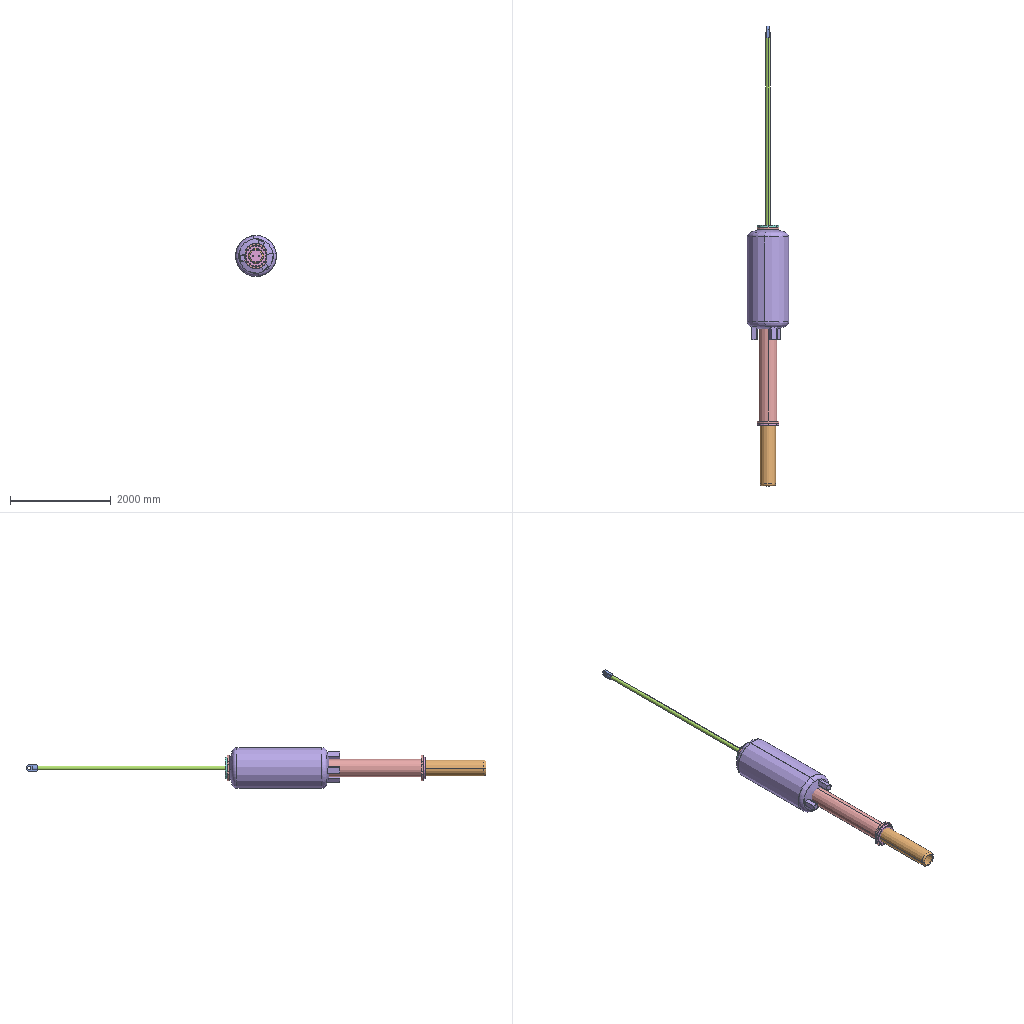Assembly | SolidWorks | 8 different items | 8 placed | box 820 x 9150 x 811 mm
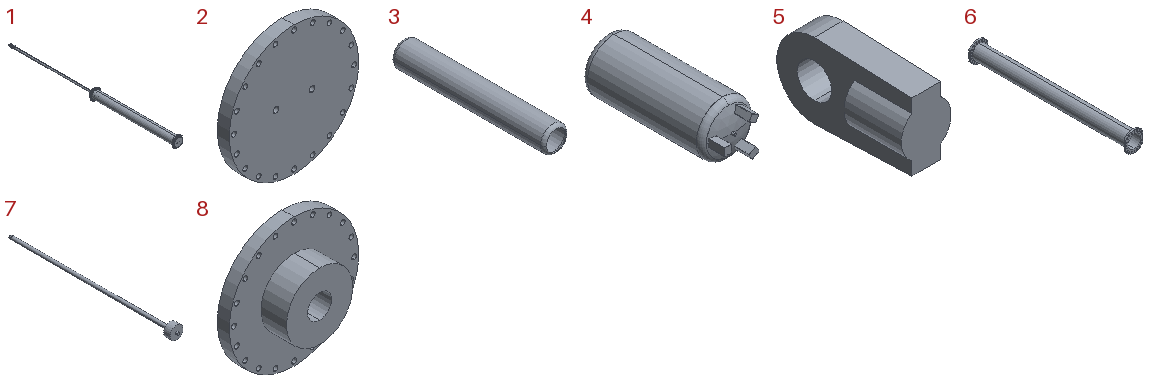Parts list (item | name | quantity | parent item | size | volume | features):
1 | (subassembly) | x1 | - | 430 x 7940 x 500 mm | 118465074 mm3 | -
2 | - | x1 | in 1 | 430 x 40 x 430 mm | 5625273 mm3 | features HoleWzd 2, Extrusion 1
3 | - | x1 | - | 310 x 1908 x 310 mm | 14769515 mm3 | features Revolution 1, Shell 1
4 | - | x1 | - | 820 x 2240 x 820 mm | 35765153 mm3 | features ICE 2, CirPattern 1, Revolution 1, Shell 1
5 | - | x1 | in 1 | 87 x 235.5 x 131 mm | 1438602 mm3 | features Extrusion 1, ICE 1
6 | - | x1 | in 1 | 430 x 3897 x 500 mm | 70114702 mm3 | features Extrusion 1, HoleWzd 1, ICE 1, LPattern 1
7 | - | x1 | in 1 | 320 x 4176 x 320 mm | 32834670 mm3 | features Revolution 1
8 | - | x1 | in 1 | 430 x 125 x 430 mm | 8451827 mm3 | features HoleWzd 2, Extrusion 1, ICE 1
Mates (type | each side: item.copy, entity, surface, feature):
In the top assembly
Coincident | 3.1 plane | assembly plane
Concentric | 6.1 face cylinder Boss-Extrude2 | 4.1 face cylinder Revolve1
Concentric | 6.1 face cylinder Boss-Extrude2 | 3.1 face cylinder Revolve1
Tangent | 2.1 face plane Boss-Extrude1 | 3.1 face sphere Revolve1
Coordinate | 1.1 select_type:25 | assembly select_type:11
In subassembly 1
Concentric | 6.2 face cylinder Boss-Extrude2 | 7.1 face cylinder Revolve1
Concentric | 6.2 face cylinder Boss-Extrude1 | 2.2 face cylinder Boss-Extrude1
Concentric | 6.2 face cylinder Ø16.0 (16) Diameter Hole1 | 2.2 face cylinder Ø16.0 (16) Diameter Hole1
Coincident | 6.2 face plane Boss-Extrude1 | 2.2 face plane Boss-Extrude1
Concentric | 6.2 face cylinder LPattern1 | 8.1 face cylinder Boss-Extrude1
Coincident | 6.2 face plane LPattern1 | 8.1 face plane Boss-Extrude1
Concentric | 6.2 face cylinder LPattern1 | 8.1 face cylinder Ø16.0 (16) Diameter Hole1
Concentric | 5.1 face cylinder Boss-Extrude2 | 7.1 face cylinder Revolve1
Coincident | 5.1 face plane Boss-Extrude1 | 7.1 face plane Revolve1
Parallel | 5.1 face plane Boss-Extrude1 | 1.2 plane